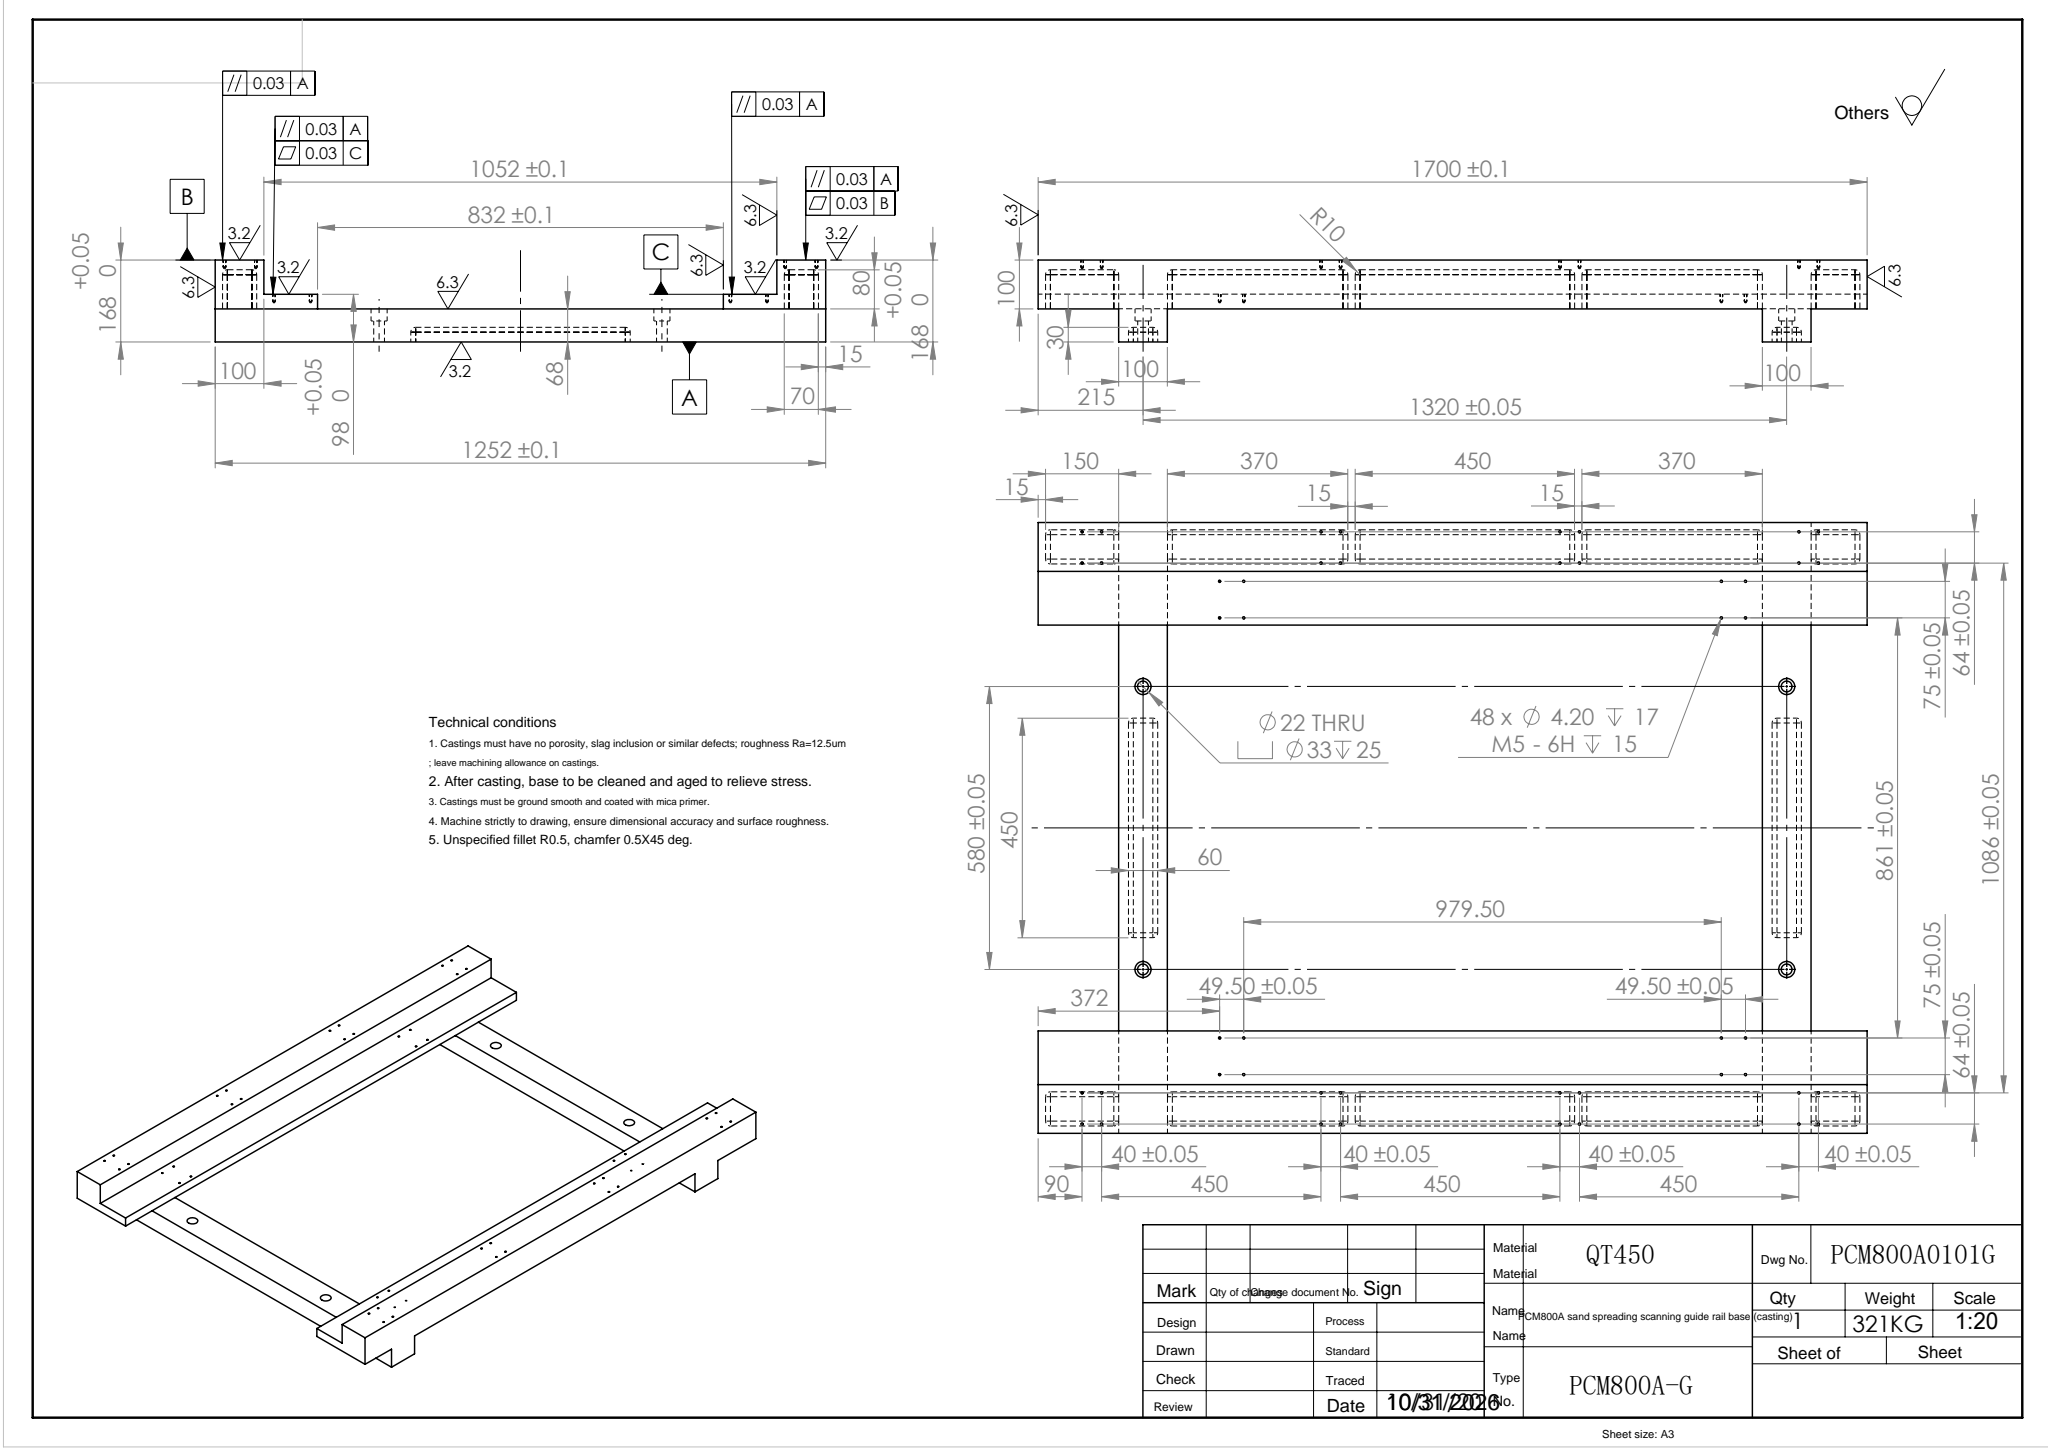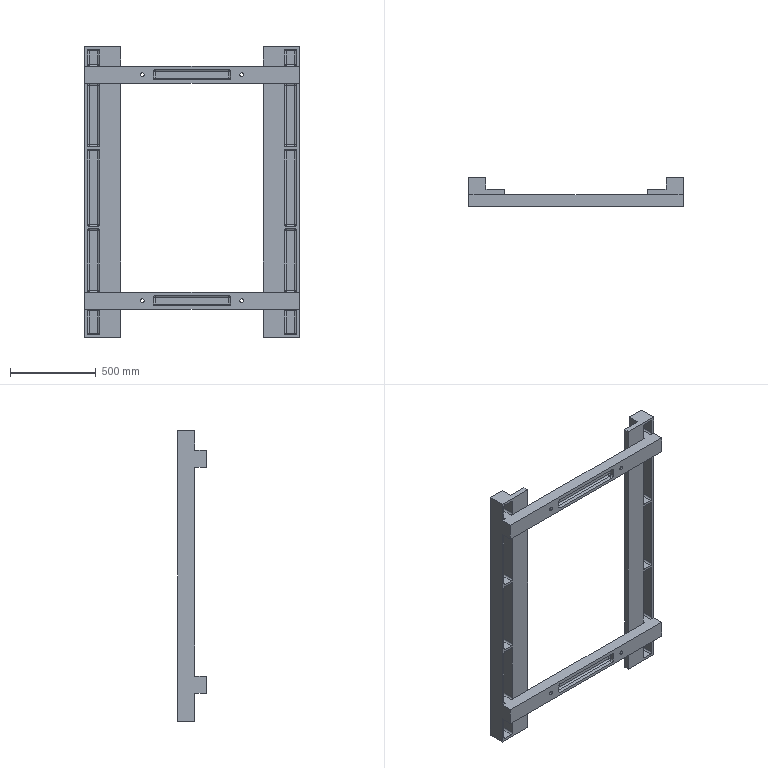Part | SolidWorks | features ICE 4, HoleWzd 3, Fillet 2, Shell 2, Extrusion 1, MirrorPattern 1 | 1 solid | 436 faces | box 1252 x 168 x 1700 mm | volume 44599924 mm3 | cylinder 208 | cone 96 | plane 84 | sphere 48 | commonest cylinder face diameters 4.2 x96 20 x96 22 x8 33 x8